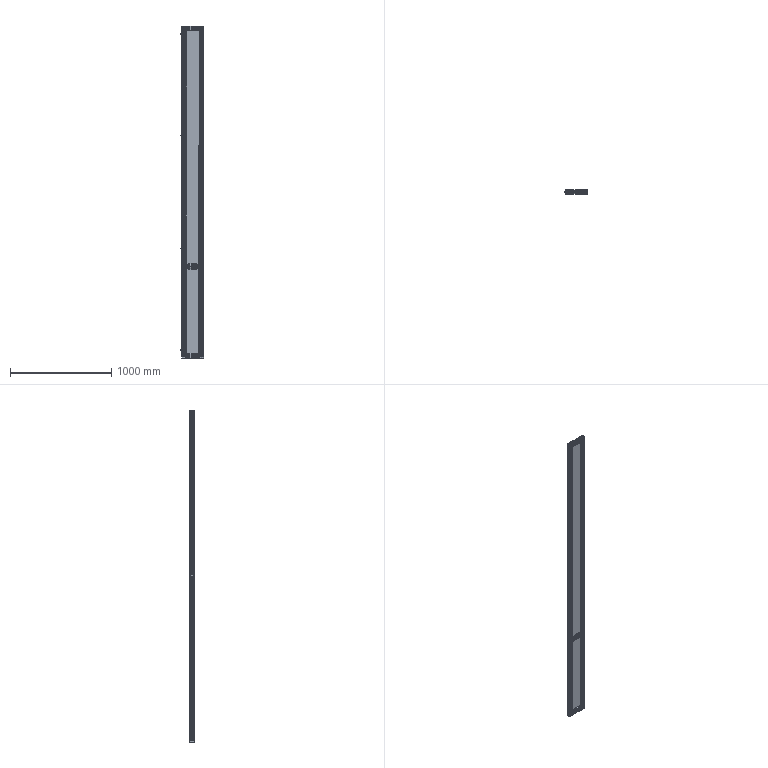Part | SolidWorks | features ReferencePattern 12, LocalLPattern 4 | 67 solids | 3410 faces | volume 6905268 mm3 | plane 2303 | cylinder 935 | cone 140 | spline 32 | commonest cylinder face diameters 0.562 x120 5 x104 6.8 x103 11 x56 2 x54 8 x48